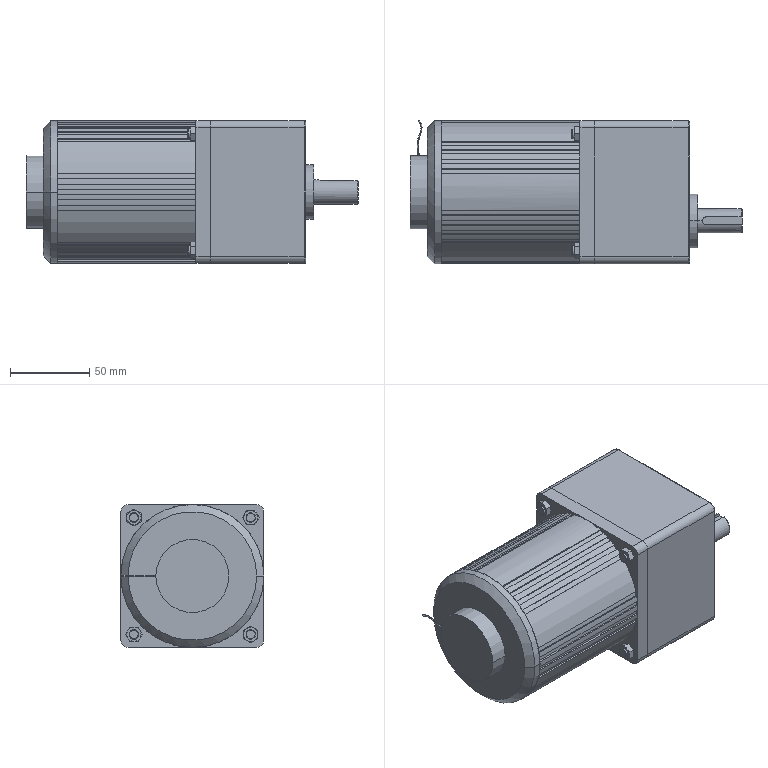Part | SolidWorks | features ICE 12, Fillet 4, CirPattern 3, Chamfer 2, Revolution 2, Sweep 1 | 3 solids | 344 faces | box 209 x 90.466 x 90 mm | volume 815406 mm3 | plane 191 | cylinder 100 | cone 39 | torus 12 | spline 2 | commonest cylinder face diameters 90 x27 88 x24 9 x16 6 x8 9.2 x8 1.8 x4